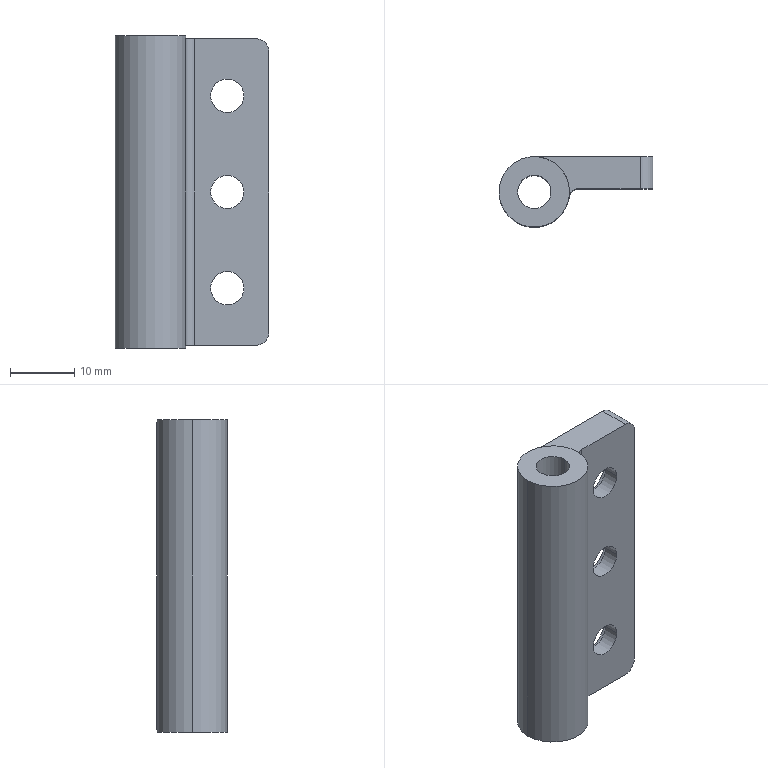Part | SolidWorks | features BaseBody 1 | 1 solid | 29 faces | box 24 x 11 x 48.8 mm | volume 6157 mm3 | cylinder 19 | plane 10 | commonest cylinder face diameters 5.2 x8 11 x8 4 x2 3 x1
STEP:
#1=CARTESIAN_POINT('',(-3.9,-5.,15.));
#2=VERTEX_POINT('',#1);
#3=CARTESIAN_POINT('',(-3.9,-2.5,15.));
#4=VERTEX_POINT('',#3);
#5=CARTESIAN_POINT('',(-3.9,-12.5,15.));
#6=DIRECTION('',(0.,1.,0.));
#7=VECTOR('',#6,1000.);
#8=LINE('',#5,#7);
#9=EDGE_CURVE('',#2,#4,#8,.T.);
#10=ORIENTED_EDGE('',*,*,#9,.F.);
#11=CARTESIAN_POINT('',(-9.1,-5.,15.));
#12=VERTEX_POINT('',#11);
#13=CARTESIAN_POINT('',(-6.5,-5.,15.));
#14=DIRECTION('',(0.,1.,0.));
#15=DIRECTION('',(-1.,0.,0.));
#16=AXIS2_PLACEMENT_3D('',#13,#14,#15);
#17=CIRCLE('',#16,2.6);
#18=EDGE_CURVE('',#12,#2,#17,.T.);
#19=ORIENTED_EDGE('',*,*,#18,.F.);
#20=CARTESIAN_POINT('',(-9.1,-2.5,15.));
#21=VERTEX_POINT('',#20);
#22=CARTESIAN_POINT('',(-9.1,-12.5,15.));
#23=DIRECTION('',(0.,1.,0.));
#24=VECTOR('',#23,1000.);
#25=LINE('',#22,#24);
#26=EDGE_CURVE('',#12,#21,#25,.T.);
#27=ORIENTED_EDGE('',*,*,#26,.T.);
#28=CARTESIAN_POINT('',(-6.5,-2.5,15.));
#29=DIRECTION('',(0.,1.,0.));
#30=DIRECTION('',(-1.,0.,0.));
#31=AXIS2_PLACEMENT_3D('',#28,#29,#30);
#32=CIRCLE('',#31,2.6);
#33=EDGE_CURVE('',#21,#4,#32,.T.);
#34=ORIENTED_EDGE('',*,*,#33,.T.);
#35=EDGE_LOOP('',(#10,#19,#27,#34));
#36=FACE_OUTER_BOUND('',#35,.T.);
#37=CARTESIAN_POINT('',(-6.5,-12.5,15.));
#38=DIRECTION('',(0.,1.,0.));
#39=DIRECTION('',(-1.,0.,0.));
#40=AXIS2_PLACEMENT_3D('',#37,#38,#39);
#41=CYLINDRICAL_SURFACE('',#40,2.6);
#42=ADVANCED_FACE('',(#36),#41,.F.);
#43=CARTESIAN_POINT('',(-3.9,-5.,0.));
#44=VERTEX_POINT('',#43);
#45=CARTESIAN_POINT('',(-3.9,-2.5,0.));
#46=VERTEX_POINT('',#45);
#47=CARTESIAN_POINT('',(-3.9,-12.5,0.));
#48=DIRECTION('',(0.,1.,0.));
#49=VECTOR('',#48,1000.);
#50=LINE('',#47,#49);
#51=EDGE_CURVE('',#44,#46,#50,.T.);
#52=ORIENTED_EDGE('',*,*,#51,.F.);
#53=CARTESIAN_POINT('',(-9.1,-5.,0.));
#54=VERTEX_POINT('',#53);
#55=CARTESIAN_POINT('',(-6.5,-5.,0.));
#56=DIRECTION('',(0.,1.,0.));
#57=DIRECTION('',(-1.,0.,0.));
#58=AXIS2_PLACEMENT_3D('',#55,#56,#57);
#59=CIRCLE('',#58,2.6);
#60=EDGE_CURVE('',#54,#44,#59,.T.);
#61=ORIENTED_EDGE('',*,*,#60,.F.);
#62=CARTESIAN_POINT('',(-9.1,-2.5,0.));
#63=VERTEX_POINT('',#62);
#64=CARTESIAN_POINT('',(-9.1,-12.5,0.));
#65=DIRECTION('',(0.,1.,0.));
#66=VECTOR('',#65,1000.);
#67=LINE('',#64,#66);
#68=EDGE_CURVE('',#54,#63,#67,.T.);
#69=ORIENTED_EDGE('',*,*,#68,.T.);
#70=CARTESIAN_POINT('',(-6.5,-2.5,0.));
#71=DIRECTION('',(0.,1.,0.));
#72=DIRECTION('',(-1.,0.,0.));
#73=AXIS2_PLACEMENT_3D('',#70,#71,#72);
#74=CIRCLE('',#73,2.6);
#75=EDGE_CURVE('',#63,#46,#74,.T.);
#76=ORIENTED_EDGE('',*,*,#75,.T.);
#77=EDGE_LOOP('',(#52,#61,#69,#76));
#78=FACE_OUTER_BOUND('',#77,.T.);
#79=CARTESIAN_POINT('',(-6.5,-12.5,0.));
#80=DIRECTION('',(0.,1.,0.));
#81=DIRECTION('',(-1.,0.,0.));
#82=AXIS2_PLACEMENT_3D('',#79,#80,#81);
#83=CYLINDRICAL_SURFACE('',#82,2.6);
#84=ADVANCED_FACE('',(#78),#83,.F.);
#85=CARTESIAN_POINT('',(-3.9,-5.,-15.));
#86=VERTEX_POINT('',#85);
#87=CARTESIAN_POINT('',(-3.9,-2.5,-15.));
#88=VERTEX_POINT('',#87);
#89=CARTESIAN_POINT('',(-3.9,-12.5,-15.));
#90=DIRECTION('',(0.,1.,0.));
#91=VECTOR('',#90,1000.);
#92=LINE('',#89,#91);
#93=EDGE_CURVE('',#86,#88,#92,.T.);
#94=ORIENTED_EDGE('',*,*,#93,.F.);
#95=CARTESIAN_POINT('',(-9.1,-5.,-15.));
#96=VERTEX_POINT('',#95);
#97=CARTESIAN_POINT('',(-6.5,-5.,-15.));
#98=DIRECTION('',(0.,1.,0.));
#99=DIRECTION('',(-1.,0.,0.));
#100=AXIS2_PLACEMENT_3D('',#97,#98,#99);
#101=CIRCLE('',#100,2.6);
#102=EDGE_CURVE('',#96,#86,#101,.T.);
#103=ORIENTED_EDGE('',*,*,#102,.F.);
#104=CARTESIAN_POINT('',(-9.1,-2.5,-15.));
#105=VERTEX_POINT('',#104);
#106=CARTESIAN_POINT('',(-9.1,-12.5,-15.));
#107=DIRECTION('',(0.,1.,0.));
#108=VECTOR('',#107,1000.);
#109=LINE('',#106,#108);
#110=EDGE_CURVE('',#96,#105,#109,.T.);
#111=ORIENTED_EDGE('',*,*,#110,.T.);
#112=CARTESIAN_POINT('',(-6.5,-2.5,-15.));
#113=DIRECTION('',(0.,1.,0.));
#114=DIRECTION('',(-1.,0.,0.));
#115=AXIS2_PLACEMENT_3D('',#112,#113,#114);
#116=CIRCLE('',#115,2.6);
#117=EDGE_CURVE('',#105,#88,#116,.T.);
#118=ORIENTED_EDGE('',*,*,#117,.T.);
#119=EDGE_LOOP('',(#94,#103,#111,#118));
#120=FACE_OUTER_BOUND('',#119,.T.);
#121=CARTESIAN_POINT('',(-6.5,-12.5,-15.));
#122=DIRECTION('',(0.,1.,0.));
#123=DIRECTION('',(-1.,0.,0.));
#124=AXIS2_PLACEMENT_3D('',#121,#122,#123);
#125=CYLINDRICAL_SURFACE('',#124,2.6);
#126=ADVANCED_FACE('',(#120),#125,.F.);
#127=ORIENTED_EDGE('',*,*,#33,.F.);
#128=CARTESIAN_POINT('',(-6.5,-2.5,15.));
#129=DIRECTION('',(0.,1.,0.));
#130=DIRECTION('',(-1.,0.,0.));
#131=AXIS2_PLACEMENT_3D('',#128,#129,#130);
#132=CIRCLE('',#131,2.6);
#133=EDGE_CURVE('',#4,#21,#132,.T.);
#134=ORIENTED_EDGE('',*,*,#133,.F.);
#135=EDGE_LOOP('',(#127,#134));
#136=FACE_BOUND('',#135,.T.);
#137=CARTESIAN_POINT('',(-12.,-2.5,15.));
#138=VERTEX_POINT('',#137);
#139=CARTESIAN_POINT('',(-1.,-2.5,15.));
#140=VERTEX_POINT('',#139);
#141=CARTESIAN_POINT('',(-6.5,-2.5,15.));
#142=DIRECTION('',(0.,1.,0.));
#143=DIRECTION('',(1.,0.,0.));
#144=AXIS2_PLACEMENT_3D('',#141,#142,#143);
#145=CIRCLE('',#144,5.5);
#146=EDGE_CURVE('',#138,#140,#145,.T.);
#147=ORIENTED_EDGE('',*,*,#146,.T.);
#148=CARTESIAN_POINT('',(-6.5,-2.5,15.));
#149=DIRECTION('',(0.,1.,0.));
#150=DIRECTION('',(1.,0.,0.));
#151=AXIS2_PLACEMENT_3D('',#148,#149,#150);
#152=CIRCLE('',#151,5.5);
#153=EDGE_CURVE('',#140,#138,#152,.T.);
#154=ORIENTED_EDGE('',*,*,#153,.T.);
#155=EDGE_LOOP('',(#147,#154));
#156=FACE_OUTER_BOUND('',#155,.T.);
#157=CARTESIAN_POINT('',(-6.5,-2.5,15.));
#158=DIRECTION('',(0.,-1.,0.));
#159=DIRECTION('',(0.,0.,-1.));
#160=AXIS2_PLACEMENT_3D('',#157,#158,#159);
#161=PLANE('',#160);
#162=ADVANCED_FACE('',(#136,#156),#161,.F.);
#163=CARTESIAN_POINT('',(-1.,0.,15.));
#164=VERTEX_POINT('',#163);
#165=CARTESIAN_POINT('',(-1.,-2.5,15.));
#166=DIRECTION('',(0.,1.,0.));
#167=VECTOR('',#166,1000.);
#168=LINE('',#165,#167);
#169=EDGE_CURVE('',#140,#164,#168,.T.);
#170=ORIENTED_EDGE('',*,*,#169,.F.);
#171=ORIENTED_EDGE('',*,*,#146,.F.);
#172=CARTESIAN_POINT('',(-12.,0.,15.));
#173=VERTEX_POINT('',#172);
#174=CARTESIAN_POINT('',(-12.,-2.5,15.));
#175=DIRECTION('',(0.,1.,0.));
#176=VECTOR('',#175,1000.);
#177=LINE('',#174,#176);
#178=EDGE_CURVE('',#138,#173,#177,.T.);
#179=ORIENTED_EDGE('',*,*,#178,.T.);
#180=CARTESIAN_POINT('',(-6.5,0.,15.));
#181=DIRECTION('',(0.,1.,0.));
#182=DIRECTION('',(1.,0.,0.));
#183=AXIS2_PLACEMENT_3D('',#180,#181,#182);
#184=CIRCLE('',#183,5.5);
#185=EDGE_CURVE('',#173,#164,#184,.T.);
#186=ORIENTED_EDGE('',*,*,#185,.T.);
#187=EDGE_LOOP('',(#170,#171,#179,#186));
#188=FACE_OUTER_BOUND('',#187,.T.);
#189=CARTESIAN_POINT('',(-6.5,-2.5,15.));
#190=DIRECTION('',(0.,1.,0.));
#191=DIRECTION('',(-1.,0.,0.));
#192=AXIS2_PLACEMENT_3D('',#189,#190,#191);
#193=CYLINDRICAL_SURFACE('',#192,5.5);
#194=ADVANCED_FACE('',(#188),#193,.F.);
#195=ORIENTED_EDGE('',*,*,#117,.F.);
#196=CARTESIAN_POINT('',(-6.5,-2.5,-15.));
#197=DIRECTION('',(0.,1.,0.));
#198=DIRECTION('',(-1.,0.,0.));
#199=AXIS2_PLACEMENT_3D('',#196,#197,#198);
#200=CIRCLE('',#199,2.6);
#201=EDGE_CURVE('',#88,#105,#200,.T.);
#202=ORIENTED_EDGE('',*,*,#201,.F.);
#203=EDGE_LOOP('',(#195,#202));
#204=FACE_BOUND('',#203,.T.);
#205=CARTESIAN_POINT('',(-12.,-2.5,-15.));
#206=VERTEX_POINT('',#205);
#207=CARTESIAN_POINT('',(-1.,-2.5,-15.));
#208=VERTEX_POINT('',#207);
#209=CARTESIAN_POINT('',(-6.5,-2.5,-15.));
#210=DIRECTION('',(0.,1.,0.));
#211=DIRECTION('',(-1.,0.,0.));
#212=AXIS2_PLACEMENT_3D('',#209,#210,#211);
#213=CIRCLE('',#212,5.5);
#214=EDGE_CURVE('',#206,#208,#213,.T.);
#215=ORIENTED_EDGE('',*,*,#214,.T.);
#216=CARTESIAN_POINT('',(-6.5,-2.5,-15.));
#217=DIRECTION('',(0.,1.,0.));
#218=DIRECTION('',(-1.,0.,0.));
#219=AXIS2_PLACEMENT_3D('',#216,#217,#218);
#220=CIRCLE('',#219,5.5);
#221=EDGE_CURVE('',#208,#206,#220,.T.);
#222=ORIENTED_EDGE('',*,*,#221,.T.);
#223=EDGE_LOOP('',(#215,#222));
#224=FACE_OUTER_BOUND('',#223,.T.);
#225=CARTESIAN_POINT('',(-6.5,-2.5,-15.));
#226=DIRECTION('',(0.,1.,0.));
#227=DIRECTION('',(1.,0.,0.));
#228=AXIS2_PLACEMENT_3D('',#225,#226,#227);
#229=PLANE('',#228);
#230=ADVANCED_FACE('',(#204,#224),#229,.T.);
#231=CARTESIAN_POINT('',(-1.,0.,-15.));
#232=VERTEX_POINT('',#231);
#233=CARTESIAN_POINT('',(-1.,-2.5,-15.));
#234=DIRECTION('',(0.,1.,0.));
#235=VECTOR('',#234,1000.);
#236=LINE('',#233,#235);
#237=EDGE_CURVE('',#208,#232,#236,.T.);
#238=ORIENTED_EDGE('',*,*,#237,.F.);
#239=ORIENTED_EDGE('',*,*,#214,.F.);
#240=CARTESIAN_POINT('',(-12.,0.,-15.));
#241=VERTEX_POINT('',#240);
#242=CARTESIAN_POINT('',(-12.,-2.5,-15.));
#243=DIRECTION('',(0.,1.,0.));
#244=VECTOR('',#243,1000.);
#245=LINE('',#242,#244);
#246=EDGE_CURVE('',#206,#241,#245,.T.);
#247=ORIENTED_EDGE('',*,*,#246,.T.);
#248=CARTESIAN_POINT('',(-6.5,0.,-15.));
#249=DIRECTION('',(0.,1.,0.));
#250=DIRECTION('',(-1.,0.,0.));
#251=AXIS2_PLACEMENT_3D('',#248,#249,#250);
#252=CIRCLE('',#251,5.5);
#253=EDGE_CURVE('',#241,#232,#252,.T.);
#254=ORIENTED_EDGE('',*,*,#253,.T.);
#255=EDGE_LOOP('',(#238,#239,#247,#254));
#256=FACE_OUTER_BOUND('',#255,.T.);
#257=CARTESIAN_POINT('',(-6.5,-2.5,-15.));
#258=DIRECTION('',(0.,1.,0.));
#259=DIRECTION('',(-1.,0.,0.));
#260=AXIS2_PLACEMENT_3D('',#257,#258,#259);
#261=CYLINDRICAL_SURFACE('',#260,5.5);
#262=ADVANCED_FACE('',(#256),#261,.F.);
#263=ORIENTED_EDGE('',*,*,#75,.F.);
#264=CARTESIAN_POINT('',(-6.5,-2.5,0.));
#265=DIRECTION('',(0.,1.,0.));
#266=DIRECTION('',(-1.,0.,0.));
#267=AXIS2_PLACEMENT_3D('',#264,#265,#266);
#268=CIRCLE('',#267,2.6);
#269=EDGE_CURVE('',#46,#63,#268,.T.);
#270=ORIENTED_EDGE('',*,*,#269,.F.);
#271=EDGE_LOOP('',(#263,#270));
#272=FACE_BOUND('',#271,.T.);
#273=CARTESIAN_POINT('',(-12.,-2.5,0.));
#274=VERTEX_POINT('',#273);
#275=CARTESIAN_POINT('',(-1.,-2.5,0.));
#276=VERTEX_POINT('',#275);
#277=CARTESIAN_POINT('',(-6.5,-2.5,0.));
#278=DIRECTION('',(0.,1.,0.));
#279=DIRECTION('',(-1.,0.,0.));
#280=AXIS2_PLACEMENT_3D('',#277,#278,#279);
#281=CIRCLE('',#280,5.5);
#282=EDGE_CURVE('',#274,#276,#281,.T.);
#283=ORIENTED_EDGE('',*,*,#282,.T.);
#284=CARTESIAN_POINT('',(-6.5,-2.5,0.));
#285=DIRECTION('',(0.,1.,0.));
#286=DIRECTION('',(-1.,0.,0.));
#287=AXIS2_PLACEMENT_3D('',#284,#285,#286);
#288=CIRCLE('',#287,5.5);
#289=EDGE_CURVE('',#276,#274,#288,.T.);
#290=ORIENTED_EDGE('',*,*,#289,.T.);
#291=EDGE_LOOP('',(#283,#290));
#292=FACE_OUTER_BOUND('',#291,.T.);
#293=CARTESIAN_POINT('',(-6.5,-2.5,0.));
#294=DIRECTION('',(0.,1.,0.));
#295=DIRECTION('',(1.,0.,0.));
#296=AXIS2_PLACEMENT_3D('',#293,#294,#295);
#297=PLANE('',#296);
#298=ADVANCED_FACE('',(#272,#292),#297,.T.);
#299=CARTESIAN_POINT('',(-1.,0.,0.));
#300=VERTEX_POINT('',#299);
#301=CARTESIAN_POINT('',(-1.,-2.5,0.));
#302=DIRECTION('',(0.,1.,0.));
#303=VECTOR('',#302,1000.);
#304=LINE('',#301,#303);
#305=EDGE_CURVE('',#276,#300,#304,.T.);
#306=ORIENTED_EDGE('',*,*,#305,.F.);
#307=ORIENTED_EDGE('',*,*,#282,.F.);
#308=CARTESIAN_POINT('',(-12.,0.,0.));
#309=VERTEX_POINT('',#308);
#310=CARTESIAN_POINT('',(-12.,-2.5,0.));
#311=DIRECTION('',(0.,1.,0.));
#312=VECTOR('',#311,1000.);
#313=LINE('',#310,#312);
#314=EDGE_CURVE('',#274,#309,#313,.T.);
#315=ORIENTED_EDGE('',*,*,#314,.T.);
#316=CARTESIAN_POINT('',(-6.5,0.,0.));
#317=DIRECTION('',(0.,1.,0.));
#318=DIRECTION('',(-1.,0.,0.));
#319=AXIS2_PLACEMENT_3D('',#316,#317,#318);
#320=CIRCLE('',#319,5.5);
#321=EDGE_CURVE('',#309,#300,#320,.T.);
#322=ORIENTED_EDGE('',*,*,#321,.T.);
#323=EDGE_LOOP('',(#306,#307,#315,#322));
#324=FACE_OUTER_BOUND('',#323,.T.);
#325=CARTESIAN_POINT('',(-6.5,-2.5,0.));
#326=DIRECTION('',(0.,1.,0.));
#327=DIRECTION('',(-1.,0.,0.));
#328=AXIS2_PLACEMENT_3D('',#325,#326,#327);
#329=CYLINDRICAL_SURFACE('',#328,5.5);
#330=ADVANCED_FACE('',(#324),#329,.F.);
#331=CARTESIAN_POINT('',(0.,-5.,21.9));
#332=VERTEX_POINT('',#331);
#333=CARTESIAN_POINT('',(-2.,-5.,23.9));
#334=VERTEX_POINT('',#333);
#335=CARTESIAN_POINT('',(-2.,-5.,21.9));
#336=DIRECTION('',(0.,-1.,0.));
#337=DIRECTION('',(-1.,0.,0.));
#338=AXIS2_PLACEMENT_3D('',#335,#336,#337);
#339=CIRCLE('',#338,2.);
#340=EDGE_CURVE('',#332,#334,#339,.T.);
#341=ORIENTED_EDGE('',*,*,#340,.F.);
#342=CARTESIAN_POINT('',(0.,0.,21.9));
#343=VERTEX_POINT('',#342);
#344=CARTESIAN_POINT('',(0.,-5.,21.9));
#345=DIRECTION('',(0.,-1.,0.));
#346=VECTOR('',#345,1000.);
#347=LINE('',#344,#346);
#348=EDGE_CURVE('',#343,#332,#347,.T.);
#349=ORIENTED_EDGE('',*,*,#348,.F.);
#350=CARTESIAN_POINT('',(-2.,0.,23.9));
#351=VERTEX_POINT('',#350);
#352=CARTESIAN_POINT('',(-2.,0.,21.9));
#353=DIRECTION('',(0.,1.,0.));
#354=DIRECTION('',(1.,0.,0.));
#355=AXIS2_PLACEMENT_3D('',#352,#353,#354);
#356=CIRCLE('',#355,2.);
#357=EDGE_CURVE('',#351,#343,#356,.T.);
#358=ORIENTED_EDGE('',*,*,#357,.F.);
#359=CARTESIAN_POINT('',(-2.,0.,23.9));
#360=DIRECTION('',(0.,1.,0.));
#361=VECTOR('',#360,1000.);
#362=LINE('',#359,#361);
#363=EDGE_CURVE('',#334,#351,#362,.T.);
#364=ORIENTED_EDGE('',*,*,#363,.F.);
#365=EDGE_LOOP('',(#341,#349,#358,#364));
#366=FACE_OUTER_BOUND('',#365,.T.);
#367=CARTESIAN_POINT('',(-2.,-5.5,21.9));
#368=DIRECTION('',(0.,-1.,0.));
#369=DIRECTION('',(1.,0.,0.));
#370=AXIS2_PLACEMENT_3D('',#367,#368,#369);
#371=CYLINDRICAL_SURFACE('',#370,2.);
#372=ADVANCED_FACE('',(#366),#371,.T.);
#373=CARTESIAN_POINT('',(-2.,-5.,-23.9));
#374=VERTEX_POINT('',#373);
#375=CARTESIAN_POINT('',(0.,-5.,-21.9));
#376=VERTEX_POINT('',#375);
#377=CARTESIAN_POINT('',(-2.,-5.,-21.9));
#378=DIRECTION('',(0.,-1.,0.));
#379=DIRECTION('',(-1.,0.,0.));
#380=AXIS2_PLACEMENT_3D('',#377,#378,#379);
#381=CIRCLE('',#380,2.);
#382=EDGE_CURVE('',#374,#376,#381,.T.);
#383=ORIENTED_EDGE('',*,*,#382,.F.);
#384=CARTESIAN_POINT('',(-2.,0.,-23.9));
#385=VERTEX_POINT('',#384);
#386=CARTESIAN_POINT('',(-2.,-5.5,-23.9));
#387=DIRECTION('',(0.,-1.,0.));
#388=VECTOR('',#387,1000.);
#389=LINE('',#386,#388);
#390=EDGE_CURVE('',#385,#374,#389,.T.);
#391=ORIENTED_EDGE('',*,*,#390,.F.);
#392=CARTESIAN_POINT('',(0.,0.,-21.9));
#393=VERTEX_POINT('',#392);
#394=CARTESIAN_POINT('',(-2.,0.,-21.9));
#395=DIRECTION('',(0.,1.,0.));
#396=DIRECTION('',(1.,0.,0.));
#397=AXIS2_PLACEMENT_3D('',#394,#395,#396);
#398=CIRCLE('',#397,2.);
#399=EDGE_CURVE('',#393,#385,#398,.T.);
#400=ORIENTED_EDGE('',*,*,#399,.F.);
#401=CARTESIAN_POINT('',(0.,0.,-21.9));
#402=DIRECTION('',(0.,1.,0.));
#403=VECTOR('',#402,1000.);
#404=LINE('',#401,#403);
#405=EDGE_CURVE('',#376,#393,#404,.T.);
#406=ORIENTED_EDGE('',*,*,#405,.F.);
#407=EDGE_LOOP('',(#383,#391,#400,#406));
#408=FACE_OUTER_BOUND('',#407,.T.);
#409=CARTESIAN_POINT('',(-2.,0.,-21.9));
#410=DIRECTION('',(0.,1.,0.));
#411=DIRECTION('',(-1.,0.,0.));
#412=AXIS2_PLACEMENT_3D('',#409,#410,#411);
#413=CYLINDRICAL_SURFACE('',#412,2.);
#414=ADVANCED_FACE('',(#408),#413,.T.);
#415=CARTESIAN_POINT('',(-13.056,-6.286,23.9));
#416=VERTEX_POINT('',#415);
#417=CARTESIAN_POINT('',(-11.572,-5.,23.9));
#418=VERTEX_POINT('',#417);
#419=CARTESIAN_POINT('',(-11.572,-6.5,23.9));
#420=DIRECTION('',(0.,0.,-1.));
#421=DIRECTION('',(1.,0.,0.));
#422=AXIS2_PLACEMENT_3D('',#419,#420,#421);
#423=CIRCLE('',#422,1.5);
#424=EDGE_CURVE('',#416,#418,#423,.T.);
#425=ORIENTED_EDGE('',*,*,#424,.F.);
#426=CARTESIAN_POINT('',(-13.056,-6.286,-23.9));
#427=VERTEX_POINT('',#426);
#428=CARTESIAN_POINT('',(-13.056,-6.286,23.9));
#429=DIRECTION('',(0.,0.,1.));
#430=VECTOR('',#429,1000.);
#431=LINE('',#428,#430);
#432=EDGE_CURVE('',#427,#416,#431,.T.);
#433=ORIENTED_EDGE('',*,*,#432,.F.);
#434=CARTESIAN_POINT('',(-11.572,-5.,-23.9));
#435=VERTEX_POINT('',#434);
#436=CARTESIAN_POINT('',(-11.572,-6.5,-23.9));
#437=DIRECTION('',(0.,0.,1.));
#438=DIRECTION('',(1.,0.,0.));
#439=AXIS2_PLACEMENT_3D('',#436,#437,#438);
#440=CIRCLE('',#439,1.5);
#441=EDGE_CURVE('',#435,#427,#440,.T.);
#442=ORIENTED_EDGE('',*,*,#441,.F.);
#443=CARTESIAN_POINT('',(-11.572,-5.,-23.9));
#444=DIRECTION('',(0.,0.,-1.));
#445=VECTOR('',#444,1000.);
#446=LINE('',#443,#445);
#447=EDGE_CURVE('',#418,#435,#446,.T.);
#448=ORIENTED_EDGE('',*,*,#447,.F.);
#449=EDGE_LOOP('',(#425,#433,#442,#448));
#450=FACE_OUTER_BOUND('',#449,.T.);
#451=CARTESIAN_POINT('',(-11.572,-6.5,23.9));
#452=DIRECTION('',(0.,0.,-1.));
#453=DIRECTION('',(-1.,0.,0.));
#454=AXIS2_PLACEMENT_3D('',#451,#452,#453);
#455=CYLINDRICAL_SURFACE('',#454,1.5);
#456=ADVANCED_FACE('',(#450),#455,.F.);
#457=CARTESIAN_POINT('',(-21.1,-5.5,-24.4));
#458=VERTEX_POINT('',#457);
#459=CARTESIAN_POINT('',(-15.9,-5.5,-24.4));
#460=VERTEX_POINT('',#459);
#461=CARTESIAN_POINT('',(-18.5,-5.5,-24.4));
#462=DIRECTION('',(0.,0.,1.));
#463=DIRECTION('',(1.,0.,0.));
#464=AXIS2_PLACEMENT_3D('',#461,#462,#463);
#465=CIRCLE('',#464,2.6);
#466=EDGE_CURVE('',#458,#460,#465,.T.);
#467=ORIENTED_EDGE('',*,*,#466,.T.);
#468=CARTESIAN_POINT('',(-18.5,-5.5,-24.4));
#469=DIRECTION('',(0.,0.,1.));
#470=DIRECTION('',(1.,0.,0.));
#471=AXIS2_PLACEMENT_3D('',#468,#469,#470);
#472=CIRCLE('',#471,2.6);
#473=EDGE_CURVE('',#460,#458,#472,.T.);
#474=ORIENTED_EDGE('',*,*,#473,.T.);
#475=EDGE_LOOP('',(#467,#474));
#476=FACE_BOUND('',#475,.T.);
#477=CARTESIAN_POINT('',(-24.,-5.5,-24.4));
#478=VERTEX_POINT('',#477);
#479=CARTESIAN_POINT('',(-13.,-5.5,-24.4));
#480=VERTEX_POINT('',#479);
#481=CARTESIAN_POINT('',(-18.5,-5.5,-24.4));
#482=DIRECTION('',(0.,0.,1.));
#483=DIRECTION('',(1.,0.,0.));
#484=AXIS2_PLACEMENT_3D('',#481,#482,#483);
#485=CIRCLE('',#484,5.5);
#486=EDGE_CURVE('',#478,#480,#485,.T.);
#487=ORIENTED_EDGE('',*,*,#486,.F.);
#488=CARTESIAN_POINT('',(-18.5,-5.5,-24.4));
#489=DIRECTION('',(0.,0.,1.));
#490=DIRECTION('',(1.,0.,0.));
#491=AXIS2_PLACEMENT_3D('',#488,#489,#490);
#492=CIRCLE('',#491,5.5);
#493=EDGE_CURVE('',#480,#478,#492,.T.);
#494=ORIENTED_EDGE('',*,*,#493,.F.);
#495=EDGE_LOOP('',(#487,#494));
#496=FACE_OUTER_BOUND('',#495,.T.);
#497=CARTESIAN_POINT('',(-18.5,-5.5,-24.4));
#498=DIRECTION('',(0.,0.,-1.));
#499=DIRECTION('',(-1.,0.,0.));
#500=AXIS2_PLACEMENT_3D('',#497,#498,#499);
#501=PLANE('',#500);
#502=ADVANCED_FACE('',(#476,#496),#501,.T.);
#503=CARTESIAN_POINT('',(-21.1,-5.5,24.4));
#504=VERTEX_POINT('',#503);
#505=CARTESIAN_POINT('',(-15.9,-5.5,24.4));
#506=VERTEX_POINT('',#505);
#507=CARTESIAN_POINT('',(-18.5,-5.5,24.4));
#508=DIRECTION('',(0.,0.,1.));
#509=DIRECTION('',(1.,0.,0.));
#510=AXIS2_PLACEMENT_3D('',#507,#508,#509);
#511=CIRCLE('',#510,2.6);
#512=EDGE_CURVE('',#504,#506,#511,.T.);
#513=ORIENTED_EDGE('',*,*,#512,.F.);
#514=CARTESIAN_POINT('',(-18.5,-5.5,24.4));
#515=DIRECTION('',(0.,0.,1.));
#516=DIRECTION('',(1.,0.,0.));
#517=AXIS2_PLACEMENT_3D('',#514,#515,#516);
#518=CIRCLE('',#517,2.6);
#519=EDGE_CURVE('',#506,#504,#518,.T.);
#520=ORIENTED_EDGE('',*,*,#519,.F.);
#521=EDGE_LOOP('',(#513,#520));
#522=FACE_BOUND('',#521,.T.);
#523=CARTESIAN_POINT('',(-24.,-5.5,24.4));
#524=VERTEX_POINT('',#523);
#525=CARTESIAN_POINT('',(-13.,-5.5,24.4));
#526=VERTEX_POINT('',#525);
#527=CARTESIAN_POINT('',(-18.5,-5.5,24.4));
#528=DIRECTION('',(0.,0.,1.));
#529=DIRECTION('',(1.,0.,0.));
#530=AXIS2_PLACEMENT_3D('',#527,#528,#529);
#531=CIRCLE('',#530,5.5);
#532=EDGE_CURVE('',#524,#526,#531,.T.);
#533=ORIENTED_EDGE('',*,*,#532,.T.);
#534=CARTESIAN_POINT('',(-18.5,-5.5,24.4));
#535=DIRECTION('',(0.,0.,1.));
#536=DIRECTION('',(1.,0.,0.));
#537=AXIS2_PLACEMENT_3D('',#534,#535,#536);
#538=CIRCLE('',#537,5.5);
#539=EDGE_CURVE('',#526,#524,#538,.T.);
#540=ORIENTED_EDGE('',*,*,#539,.T.);
#541=EDGE_LOOP('',(#533,#540));
#542=FACE_OUTER_BOUND('',#541,.T.);
#543=CARTESIAN_POINT('',(-18.5,-5.5,24.4));
#544=DIRECTION('',(0.,0.,1.));
#545=DIRECTION('',(0.,-1.,0.));
#546=AXIS2_PLACEMENT_3D('',#543,#544,#545);
#547=PLANE('',#546);
#548=ADVANCED_FACE('',(#522,#542),#547,.T.);
#549=CARTESIAN_POINT('',(-15.9,-5.5,23.9));
#550=DIRECTION('',(0.,0.,-1.));
#551=VECTOR('',#550,1000.);
#552=LINE('',#549,#551);
#553=EDGE_CURVE('',#506,#460,#552,.T.);
#554=ORIENTED_EDGE('',*,*,#553,.F.);
#555=ORIENTED_EDGE('',*,*,#519,.T.);
#556=CARTESIAN_POINT('',(-21.1,-5.5,23.9));
#557=DIRECTION('',(0.,0.,-1.));
#558=VECTOR('',#557,1000.);
#559=LINE('',#556,#558);
#560=EDGE_CURVE('',#504,#458,#559,.T.);
#561=ORIENTED_EDGE('',*,*,#560,.T.);
#562=ORIENTED_EDGE('',*,*,#473,.F.);
#563=EDGE_LOOP('',(#554,#555,#561,#562));
#564=FACE_OUTER_BOUND('',#563,.T.);
#565=CARTESIAN_POINT('',(-18.5,-5.5,23.9));
#566=DIRECTION('',(0.,0.,-1.));
#567=DIRECTION('',(-1.,0.,0.));
#568=AXIS2_PLACEMENT_3D('',#565,#566,#567);
#569=CYLINDRICAL_SURFACE('',#568,2.6);
#570=ADVANCED_FACE('',(#564),#569,.F.);
#571=CARTESIAN_POINT('',(0.,-5.,23.9));
#572=DIRECTION('',(0.,0.,-1.));
#573=VECTOR('',#572,1000.);
#574=LINE('',#571,#573);
#575=EDGE_CURVE('',#332,#376,#574,.T.);
#576=ORIENTED_EDGE('',*,*,#575,.T.);
#577=ORIENTED_EDGE('',*,*,#405,.T.);
#578=CARTESIAN_POINT('',(0.,0.,23.9));
#579=DIRECTION('',(0.,0.,-1.));
#580=VECTOR('',#579,1000.);
#581=LINE('',#578,#580);
#582=EDGE_CURVE('',#343,#393,#581,.T.);
#583=ORIENTED_EDGE('',*,*,#582,.F.);
#584=ORIENTED_EDGE('',*,*,#348,.T.);
#585=EDGE_LOOP('',(#576,#577,#583,#584));
#586=FACE_OUTER_BOUND('',#585,.T.);
#587=CARTESIAN_POINT('',(0.,0.,23.9));
#588=DIRECTION('',(-1.,0.,0.));
#589=DIRECTION('',(0.,1.,0.));
#590=AXIS2_PLACEMENT_3D('',#587,#588,#589);
#591=PLANE('',#590);
#592=ADVANCED_FACE('',(#586),#591,.F.);
#593=ORIENTED_EDGE('',*,*,#102,.T.);
#594=CARTESIAN_POINT('',(-6.5,-5.,-15.));
#595=DIRECTION('',(0.,1.,0.));
#596=DIRECTION('',(-1.,0.,0.));
#597=AXIS2_PLACEMENT_3D('',#594,#595,#596);
#598=CIRCLE('',#597,2.6);
#599=EDGE_CURVE('',#86,#96,#598,.T.);
#600=ORIENTED_EDGE('',*,*,#599,.T.);
#601=EDGE_LOOP('',(#593,#600));
#602=FACE_BOUND('',#601,.T.);
#603=ORIENTED_EDGE('',*,*,#60,.T.);
#604=CARTESIAN_POINT('',(-6.5,-5.,0.));
#605=DIRECTION('',(0.,1.,0.));
#606=DIRECTION('',(-1.,0.,0.));
#607=AXIS2_PLACEMENT_3D('',#604,#605,#606);
#608=CIRCLE('',#607,2.6);
#609=EDGE_CURVE('',#44,#54,#608,.T.);
#610=ORIENTED_EDGE('',*,*,#609,.T.);
#611=EDGE_LOOP('',(#603,#610));
#612=FACE_BOUND('',#611,.T.);
#613=ORIENTED_EDGE('',*,*,#18,.T.);
#614=CARTESIAN_POINT('',(-6.5,-5.,15.));
#615=DIRECTION('',(0.,1.,0.));
#616=DIRECTION('',(-1.,0.,0.));
#617=AXIS2_PLACEMENT_3D('',#614,#615,#616);
#618=CIRCLE('',#617,2.6);
#619=EDGE_CURVE('',#2,#12,#618,.T.);
#620=ORIENTED_EDGE('',*,*,#619,.T.);
#621=EDGE_LOOP('',(#613,#620));
#622=FACE_BOUND('',#621,.T.);
#623=CARTESIAN_POINT('',(0.,-5.,-23.9));
#624=DIRECTION('',(1.,0.,0.));
#625=VECTOR('',#624,1000.);
#626=LINE('',#623,#625);
#627=EDGE_CURVE('',#435,#374,#626,.T.);
#628=ORIENTED_EDGE('',*,*,#627,.T.);
#629=ORIENTED_EDGE('',*,*,#382,.T.);
#630=ORIENTED_EDGE('',*,*,#575,.F.);
#631=ORIENTED_EDGE('',*,*,#340,.T.);
#632=CARTESIAN_POINT('',(0.,-5.,23.9));
#633=DIRECTION('',(1.,0.,0.));
#634=VECTOR('',#633,1000.);
#635=LINE('',#632,#634);
#636=EDGE_CURVE('',#418,#334,#635,.T.);
#637=ORIENTED_EDGE('',*,*,#636,.F.);
#638=ORIENTED_EDGE('',*,*,#447,.T.);
#639=EDGE_LOOP('',(#628,#629,#630,#631,#637,#638));
#640=FACE_OUTER_BOUND('',#639,.T.);
#641=CARTESIAN_POINT('',(0.,-5.,23.9));
#642=DIRECTION('',(0.,1.,0.));
#643=DIRECTION('',(1.,0.,0.));
#644=AXIS2_PLACEMENT_3D('',#641,#642,#643);
#645=PLANE('',#644);
#646=ADVANCED_FACE('',(#602,#612,#622,#640),#645,.F.);
#647=CARTESIAN_POINT('',(-13.,-5.5,23.9));
#648=VERTEX_POINT('',#647);
#649=CARTESIAN_POINT('',(-13.,-5.5,23.9));
#650=DIRECTION('',(0.,0.,-1.));
#651=VECTOR('',#650,1000.);
#652=LINE('',#649,#651);
#653=EDGE_CURVE('',#526,#648,#652,.T.);
#654=ORIENTED_EDGE('',*,*,#653,.F.);
#655=ORIENTED_EDGE('',*,*,#532,.F.);
#656=CARTESIAN_POINT('',(-24.,-5.5,23.9));
#657=DIRECTION('',(0.,0.,-1.));
#658=VECTOR('',#657,1000.);
#659=LINE('',#656,#658);
#660=EDGE_CURVE('',#524,#478,#659,.T.);
#661=ORIENTED_EDGE('',*,*,#660,.T.);
#662=ORIENTED_EDGE('',*,*,#486,.T.);
#663=CARTESIAN_POINT('',(-13.,-5.5,-23.9));
#664=VERTEX_POINT('',#663);
#665=CARTESIAN_POINT('',(-13.,-5.5,23.9));
#666=DIRECTION('',(0.,0.,-1.));
#667=VECTOR('',#666,1000.);
#668=LINE('',#665,#667);
#669=EDGE_CURVE('',#664,#480,#668,.T.);
#670=ORIENTED_EDGE('',*,*,#669,.F.);
#671=CARTESIAN_POINT('',(-18.5,-5.5,-23.9));
#672=DIRECTION('',(0.,0.,1.));
#673=DIRECTION('',(1.,0.,0.));
#674=AXIS2_PLACEMENT_3D('',#671,#672,#673);
#675=CIRCLE('',#674,5.5);
#676=EDGE_CURVE('',#427,#664,#675,.T.);
#677=ORIENTED_EDGE('',*,*,#676,.F.);
#678=ORIENTED_EDGE('',*,*,#432,.T.);
#679=CARTESIAN_POINT('',(-18.5,-5.5,23.9));
#680=DIRECTION('',(0.,0.,1.));
#681=DIRECTION('',(1.,0.,0.));
#682=AXIS2_PLACEMENT_3D('',#679,#680,#681);
#683=CIRCLE('',#682,5.5);
#684=EDGE_CURVE('',#416,#648,#683,.T.);
#685=ORIENTED_EDGE('',*,*,#684,.T.);
#686=EDGE_LOOP('',(#654,#655,#661,#662,#670,#677,#678,#685));
#687=FACE_OUTER_BOUND('',#686,.T.);
#688=CARTESIAN_POINT('',(-18.5,-5.5,23.9));
#689=DIRECTION('',(0.,0.,-1.));
#690=DIRECTION('',(-1.,0.,0.));
#691=AXIS2_PLACEMENT_3D('',#688,#689,#690);
#692=CYLINDRICAL_SURFACE('',#691,5.5);
#693=ADVANCED_FACE('',(#687),#692,.T.);
#694=ORIENTED_EDGE('',*,*,#321,.F.);
#695=CARTESIAN_POINT('',(-6.5,0.,0.));
#696=DIRECTION('',(0.,1.,0.));
#697=DIRECTION('',(-1.,0.,0.));
#698=AXIS2_PLACEMENT_3D('',#695,#696,#697);
#699=CIRCLE('',#698,5.5);
#700=EDGE_CURVE('',#300,#309,#699,.T.);
#701=ORIENTED_EDGE('',*,*,#700,.F.);
#702=EDGE_LOOP('',(#694,#701));
#703=FACE_BOUND('',#702,.T.);
#704=ORIENTED_EDGE('',*,*,#253,.F.);
#705=CARTESIAN_POINT('',(-6.5,0.,-15.));
#706=DIRECTION('',(0.,1.,0.));
#707=DIRECTION('',(-1.,0.,0.));
#708=AXIS2_PLACEMENT_3D('',#705,#706,#707);
#709=CIRCLE('',#708,5.5);
#710=EDGE_CURVE('',#232,#241,#709,.T.);
#711=ORIENTED_EDGE('',*,*,#710,.F.);
#712=EDGE_LOOP('',(#704,#711));
#713=FACE_BOUND('',#712,.T.);
#714=ORIENTED_EDGE('',*,*,#185,.F.);
#715=CARTESIAN_POINT('',(-6.5,0.,15.));
#716=DIRECTION('',(0.,1.,0.));
#717=DIRECTION('',(1.,0.,0.));
#718=AXIS2_PLACEMENT_3D('',#715,#716,#717);
#719=CIRCLE('',#718,5.5);
#720=EDGE_CURVE('',#164,#173,#719,.T.);
#721=ORIENTED_EDGE('',*,*,#720,.F.);
#722=EDGE_LOOP('',(#714,#721));
#723=FACE_BOUND('',#722,.T.);
#724=ORIENTED_EDGE('',*,*,#582,.T.);
#725=ORIENTED_EDGE('',*,*,#399,.T.);
#726=CARTESIAN_POINT('',(-18.5,0.,-23.9));
#727=VERTEX_POINT('',#726);
#728=CARTESIAN_POINT('',(-18.5,0.,-23.9));
#729=DIRECTION('',(-1.,0.,0.));
#730=VECTOR('',#729,1000.);
#731=LINE('',#728,#730);
#732=EDGE_CURVE('',#385,#727,#731,.T.);
#733=ORIENTED_EDGE('',*,*,#732,.T.);
#734=CARTESIAN_POINT('',(-18.5,0.,23.9));
#735=VERTEX_POINT('',#734);
#736=CARTESIAN_POINT('',(-18.5,0.,23.9));
#737=DIRECTION('',(0.,0.,-1.));
#738=VECTOR('',#737,1000.);
#739=LINE('',#736,#738);
#740=EDGE_CURVE('',#735,#727,#739,.T.);
#741=ORIENTED_EDGE('',*,*,#740,.F.);
#742=CARTESIAN_POINT('',(-18.5,0.,23.9));
#743=DIRECTION('',(-1.,0.,0.));
#744=VECTOR('',#743,1000.);
#745=LINE('',#742,#744);
#746=EDGE_CURVE('',#351,#735,#745,.T.);
#747=ORIENTED_EDGE('',*,*,#746,.F.);
#748=ORIENTED_EDGE('',*,*,#357,.T.);
#749=EDGE_LOOP('',(#724,#725,#733,#741,#747,#748));
#750=FACE_OUTER_BOUND('',#749,.T.);
#751=CARTESIAN_POINT('',(-18.5,0.,23.9));
#752=DIRECTION('',(0.,-1.,0.));
#753=DIRECTION('',(0.,0.,-1.));
#754=AXIS2_PLACEMENT_3D('',#751,#752,#753);
#755=PLANE('',#754);
#756=ADVANCED_FACE('',(#703,#713,#723,#750),#755,.F.);
#757=ORIENTED_EDGE('',*,*,#732,.F.);
#758=ORIENTED_EDGE('',*,*,#390,.T.);
#759=ORIENTED_EDGE('',*,*,#627,.F.);
#760=ORIENTED_EDGE('',*,*,#441,.T.);
#761=ORIENTED_EDGE('',*,*,#676,.T.);
#762=CARTESIAN_POINT('',(-18.5,-5.5,-23.9));
#763=DIRECTION('',(0.,0.,1.));
#764=DIRECTION('',(1.,0.,0.));
#765=AXIS2_PLACEMENT_3D('',#762,#763,#764);
#766=CIRCLE('',#765,5.5);
#767=EDGE_CURVE('',#664,#727,#766,.T.);
#768=ORIENTED_EDGE('',*,*,#767,.T.);
#769=EDGE_LOOP('',(#757,#758,#759,#760,#761,#768));
#770=FACE_OUTER_BOUND('',#769,.T.);
#771=CARTESIAN_POINT('',(-18.5,-5.5,-23.9));
#772=DIRECTION('',(0.,0.,1.));
#773=DIRECTION('',(0.,-1.,0.));
#774=AXIS2_PLACEMENT_3D('',#771,#772,#773);
#775=PLANE('',#774);
#776=ADVANCED_FACE('',(#770),#775,.F.);
#777=ORIENTED_EDGE('',*,*,#636,.T.);
#778=ORIENTED_EDGE('',*,*,#363,.T.);
#779=ORIENTED_EDGE('',*,*,#746,.T.);
#780=CARTESIAN_POINT('',(-18.5,-5.5,23.9));
#781=DIRECTION('',(0.,0.,1.));
#782=DIRECTION('',(1.,0.,0.));
#783=AXIS2_PLACEMENT_3D('',#780,#781,#782);
#784=CIRCLE('',#783,5.5);
#785=EDGE_CURVE('',#648,#735,#784,.T.);
#786=ORIENTED_EDGE('',*,*,#785,.F.);
#787=ORIENTED_EDGE('',*,*,#684,.F.);
#788=ORIENTED_EDGE('',*,*,#424,.T.);
#789=EDGE_LOOP('',(#777,#778,#779,#786,#787,#788));
#790=FACE_OUTER_BOUND('',#789,.T.);
#791=CARTESIAN_POINT('',(-18.5,-5.5,23.9));
#792=DIRECTION('',(0.,0.,1.));
#793=DIRECTION('',(0.,-1.,0.));
#794=AXIS2_PLACEMENT_3D('',#791,#792,#793);
#795=PLANE('',#794);
#796=ADVANCED_FACE('',(#790),#795,.T.);
#797=ORIENTED_EDGE('',*,*,#539,.F.);
#798=ORIENTED_EDGE('',*,*,#653,.T.);
#799=ORIENTED_EDGE('',*,*,#785,.T.);
#800=ORIENTED_EDGE('',*,*,#740,.T.);
#801=ORIENTED_EDGE('',*,*,#767,.F.);
#802=ORIENTED_EDGE('',*,*,#669,.T.);
#803=ORIENTED_EDGE('',*,*,#493,.T.);
#804=ORIENTED_EDGE('',*,*,#660,.F.);
#805=EDGE_LOOP('',(#797,#798,#799,#800,#801,#802,#803,#804));
#806=FACE_OUTER_BOUND('',#805,.T.);
#807=CARTESIAN_POINT('',(-18.5,-5.5,23.9));
#808=DIRECTION('',(0.,0.,-1.));
#809=DIRECTION('',(-1.,0.,0.));
#810=AXIS2_PLACEMENT_3D('',#807,#808,#809);
#811=CYLINDRICAL_SURFACE('',#810,5.5);
#812=ADVANCED_FACE('',(#806),#811,.T.);
#813=ORIENTED_EDGE('',*,*,#512,.T.);
#814=ORIENTED_EDGE('',*,*,#553,.T.);
#815=ORIENTED_EDGE('',*,*,#466,.F.);
#816=ORIENTED_EDGE('',*,*,#560,.F.);
#817=EDGE_LOOP('',(#813,#814,#815,#816));
#818=FACE_OUTER_BOUND('',#817,.T.);
#819=CARTESIAN_POINT('',(-18.5,-5.5,23.9));
#820=DIRECTION('',(0.,0.,-1.));
#821=DIRECTION('',(-1.,0.,0.));
#822=AXIS2_PLACEMENT_3D('',#819,#820,#821);
#823=CYLINDRICAL_SURFACE('',#822,2.6);
#824=ADVANCED_FACE('',(#818),#823,.F.);
#825=ORIENTED_EDGE('',*,*,#289,.F.);
#826=ORIENTED_EDGE('',*,*,#305,.T.);
#827=ORIENTED_EDGE('',*,*,#700,.T.);
#828=ORIENTED_EDGE('',*,*,#314,.F.);
#829=EDGE_LOOP('',(#825,#826,#827,#828));
#830=FACE_OUTER_BOUND('',#829,.T.);
#831=CARTESIAN_POINT('',(-6.5,-2.5,0.));
#832=DIRECTION('',(0.,1.,0.));
#833=DIRECTION('',(-1.,0.,0.));
#834=AXIS2_PLACEMENT_3D('',#831,#832,#833);
#835=CYLINDRICAL_SURFACE('',#834,5.5);
#836=ADVANCED_FACE('',(#830),#835,.F.);
#837=ORIENTED_EDGE('',*,*,#221,.F.);
#838=ORIENTED_EDGE('',*,*,#237,.T.);
#839=ORIENTED_EDGE('',*,*,#710,.T.);
#840=ORIENTED_EDGE('',*,*,#246,.F.);
#841=EDGE_LOOP('',(#837,#838,#839,#840));
#842=FACE_OUTER_BOUND('',#841,.T.);
#843=CARTESIAN_POINT('',(-6.5,-2.5,-15.));
#844=DIRECTION('',(0.,1.,0.));
#845=DIRECTION('',(-1.,0.,0.));
#846=AXIS2_PLACEMENT_3D('',#843,#844,#845);
#847=CYLINDRICAL_SURFACE('',#846,5.5);
#848=ADVANCED_FACE('',(#842),#847,.F.);
#849=ORIENTED_EDGE('',*,*,#153,.F.);
#850=ORIENTED_EDGE('',*,*,#169,.T.);
#851=ORIENTED_EDGE('',*,*,#720,.T.);
#852=ORIENTED_EDGE('',*,*,#178,.F.);
#853=EDGE_LOOP('',(#849,#850,#851,#852));
#854=FACE_OUTER_BOUND('',#853,.T.);
#855=CARTESIAN_POINT('',(-6.5,-2.5,15.));
#856=DIRECTION('',(0.,1.,0.));
#857=DIRECTION('',(-1.,0.,0.));
#858=AXIS2_PLACEMENT_3D('',#855,#856,#857);
#859=CYLINDRICAL_SURFACE('',#858,5.5);
#860=ADVANCED_FACE('',(#854),#859,.F.);
#861=ORIENTED_EDGE('',*,*,#599,.F.);
#862=ORIENTED_EDGE('',*,*,#93,.T.);
#863=ORIENTED_EDGE('',*,*,#201,.T.);
#864=ORIENTED_EDGE('',*,*,#110,.F.);
#865=EDGE_LOOP('',(#861,#862,#863,#864));
#866=FACE_OUTER_BOUND('',#865,.T.);
#867=CARTESIAN_POINT('',(-6.5,-12.5,-15.));
#868=DIRECTION('',(0.,1.,0.));
#869=DIRECTION('',(-1.,0.,0.));
#870=AXIS2_PLACEMENT_3D('',#867,#868,#869);
#871=CYLINDRICAL_SURFACE('',#870,2.6);
#872=ADVANCED_FACE('',(#866),#871,.F.);
#873=ORIENTED_EDGE('',*,*,#609,.F.);
#874=ORIENTED_EDGE('',*,*,#51,.T.);
#875=ORIENTED_EDGE('',*,*,#269,.T.);
#876=ORIENTED_EDGE('',*,*,#68,.F.);
#877=EDGE_LOOP('',(#873,#874,#875,#876));
#878=FACE_OUTER_BOUND('',#877,.T.);
#879=CARTESIAN_POINT('',(-6.5,-12.5,0.));
#880=DIRECTION('',(0.,1.,0.));
#881=DIRECTION('',(-1.,0.,0.));
#882=AXIS2_PLACEMENT_3D('',#879,#880,#881);
#883=CYLINDRICAL_SURFACE('',#882,2.6);
#884=ADVANCED_FACE('',(#878),#883,.F.);
#885=ORIENTED_EDGE('',*,*,#619,.F.);
#886=ORIENTED_EDGE('',*,*,#9,.T.);
#887=ORIENTED_EDGE('',*,*,#133,.T.);
#888=ORIENTED_EDGE('',*,*,#26,.F.);
#889=EDGE_LOOP('',(#885,#886,#887,#888));
#890=FACE_OUTER_BOUND('',#889,.T.);
#891=CARTESIAN_POINT('',(-6.5,-12.5,15.));
#892=DIRECTION('',(0.,1.,0.));
#893=DIRECTION('',(-1.,0.,0.));
#894=AXIS2_PLACEMENT_3D('',#891,#892,#893);
#895=CYLINDRICAL_SURFACE('',#894,2.6);
#896=ADVANCED_FACE('',(#890),#895,.F.);
#897=CLOSED_SHELL('',(#42,#84,#126,#162,#194,#230,#262,#298,#330,#372,#414,#456,#502,#548,#570,#592,#646,#693,#756,#776,#796,#812,#824,#836,#848,#860,#872,#884,#896));
#898=MANIFOLD_SOLID_BREP('',#897);
#899=CARTESIAN_POINT('',(0.,0.,0.));
#900=DIRECTION('',(0.,0.,1.));
#901=DIRECTION('',(1.,0.,0.));
#902=AXIS2_PLACEMENT_3D('',#899,#900,#901);
#903=(LENGTH_UNIT()NAMED_UNIT(*)SI_UNIT(.MILLI.,.METRE.));
#904=UNCERTAINTY_MEASURE_WITH_UNIT(LENGTH_MEASURE(0.00001),#903,'','');
#905=(NAMED_UNIT(*)PLANE_ANGLE_UNIT()SI_UNIT($,.RADIAN.));
#906=(NAMED_UNIT(*)SI_UNIT($,.STERADIAN.)SOLID_ANGLE_UNIT());
#907=(GEOMETRIC_REPRESENTATION_CONTEXT(3)GLOBAL_UNCERTAINTY_ASSIGNED_CONTEXT((#904))GLOBAL_UNIT_ASSIGNED_CONTEXT((#903,#905,#906))REPRESENTATION_CONTEXT('',''));
#908=ADVANCED_BREP_SHAPE_REPRESENTATION('',(#898,#902),#907);